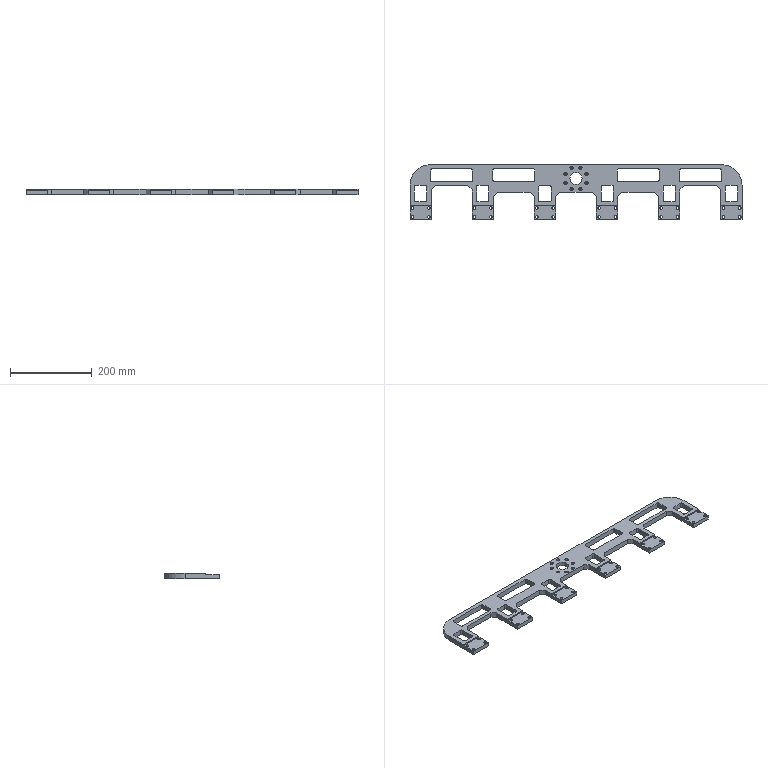NC program | NX | posted with a generic post | part box 813.6 x 134 x 13 mm
Lines 122 to 1368 of 13853:
(ZLEVEL_PROFILE_COPY_3 , TOOL : D10)
N224 T10 M6
N226 G54
N228 G17 G0 G90 X-398.182 Y53.372 S9500 M3
N230 G43 Z30. H10
N232 Z1.5
N234 G94 G1 X-396.786 Y54.924 Z1.391 F1000.
N236 X-394.726 Y56.984 Z1.238
N238 X-392.561 Y58.932 Z1.085
N240 X-390.296 Y60.762 Z0.933
N242 X-387.937 Y62.471 Z0.78
N244 X-385.492 Y64.052 Z0.627
N246 X-382.966 Y65.502 Z0.475
N248 X-380.367 Y66.817 Z0.322
N250 X-377.703 Y67.992 Z0.17
N252 X-374.98 Y69.025 Z0.017
N254 X-372.206 Y69.913 Z-0.136
N256 X-369.389 Y70.653 Z-0.288
N258 X-366.538 Y71.243 Z-0.441
N260 X-363.658 Y71.682 Z-0.594
N262 X-360.76 Y71.968 Z-0.746
N264 X-357.851 Y72.1 Z-0.899
N266 X-356.801 Z-0.954
N268 X356.8 F3500.
N270 G2 X411.9 Y17. R55.1
N272 G1 Y-67.
N274 G2 X406.8 Y-72.1 R5.1
N276 G1 X354.8
N278 G2 X349.7 Y-67. R5.1
N280 G1 Y2.888
N282 X342.687 Y9.9
N284 X266.913
N286 X259.9 Y2.888
N288 Y-67.
N290 G2 X254.8 Y-72.1 R5.1
N292 G1 X202.4
N294 G2 X197.3 Y-67. R5.1
N296 G1 Y-13.062
N298 X190.288 Y-6.05
N300 X114.512
N302 X107.5 Y-13.062
N304 Y-67.
N306 G2 X102.4 Y-72.1 R5.1
N308 G1 X50.
N310 G2 X44.9 Y-67. R5.1
N312 G1 Y-13.062
N314 X37.888 Y-6.05
N316 X-37.888
N318 X-44.9 Y-13.062
N320 Y-67.
N322 G2 X-50. Y-72.1 R5.1
N324 G1 X-102.4
N326 G2 X-107.5 Y-67. R5.1
N328 G1 Y-13.062
N330 X-114.512 Y-6.05
N332 X-190.288
N334 X-197.3 Y-13.062
N336 Y-67.
N338 G2 X-202.4 Y-72.1 R5.1
N340 G1 X-254.8
N342 G2 X-259.9 Y-67. R5.1
N344 G1 Y2.888
N346 X-266.913 Y9.9
N348 X-342.687
N350 X-349.7 Y2.888
N352 Y-67.
N354 G2 X-354.8 Y-72.1 R5.1
N356 G1 X-406.8
N358 G2 X-411.9 Y-67. R5.1
N360 G1 Y16.999
N362 G2 X-356.801 Y72.1 R55.1
N364 G1 X-302.155 Z-1.908
N366 X356.8
N368 G2 X411.9 Y17. R55.1
N370 G1 Y-67.
N372 G2 X406.8 Y-72.1 R5.1
N374 G1 X354.8
N376 G2 X349.7 Y-67. R5.1
N378 G1 Y2.888
N380 X342.687 Y9.9
N382 X266.913
N384 X259.9 Y2.888
N386 Y-67.
N388 G2 X254.8 Y-72.1 R5.1
N390 G1 X202.4
N392 G2 X197.3 Y-67. R5.1
N394 G1 Y-13.062
N396 X190.288 Y-6.05
N398 X114.512
N400 X107.5 Y-13.062
N402 Y-67.
N404 G2 X102.4 Y-72.1 R5.1
N406 G1 X50.
N408 G2 X44.9 Y-67. R5.1
N410 G1 Y-13.062
N412 X37.888 Y-6.05
N414 X-37.888
N416 X-44.9 Y-13.062
N418 Y-67.
N420 G2 X-50. Y-72.1 R5.1
N422 G1 X-102.4
N424 G2 X-107.5 Y-67. R5.1
N426 G1 Y-13.062
N428 X-114.512 Y-6.05
N430 X-190.288
N432 X-197.3 Y-13.062
N434 Y-67.
N436 G2 X-202.4 Y-72.1 R5.1
N438 G1 X-254.8
N440 G2 X-259.9 Y-67. R5.1
N442 G1 Y2.888
N444 X-266.913 Y9.9
N446 X-342.687
N448 X-349.7 Y2.888
N450 Y-67.
N452 G2 X-354.8 Y-72.1 R5.1
N454 G1 X-406.8
N456 G2 X-411.9 Y-67. R5.1
N458 G1 Y16.999
N460 G2 X-356.801 Y72.1 R55.1
N462 G1 X-302.155 Z-2.862
N464 X356.8
N466 G2 X411.9 Y17. R55.1
N468 G1 Y-67.
N470 G2 X406.8 Y-72.1 R5.1
N472 G1 X354.8
N474 G2 X349.7 Y-67. R5.1
N476 G1 Y2.888
N478 X342.687 Y9.9
N480 X266.913
N482 X259.9 Y2.888
N484 Y-67.
N486 G2 X254.8 Y-72.1 R5.1
N488 G1 X202.4
N490 G2 X197.3 Y-67. R5.1
N492 G1 Y-13.062
N494 X190.288 Y-6.05
N496 X114.512
N498 X107.5 Y-13.062
N500 Y-67.
N502 G2 X102.4 Y-72.1 R5.1
N504 G1 X50.
N506 G2 X44.9 Y-67. R5.1
N508 G1 Y-13.062
N510 X37.888 Y-6.05
N512 X-37.888
N514 X-44.9 Y-13.062
N516 Y-67.
N518 G2 X-50. Y-72.1 R5.1
N520 G1 X-102.4
N522 G2 X-107.5 Y-67. R5.1
N524 G1 Y-13.062
N526 X-114.512 Y-6.05
N528 X-190.288
N530 X-197.3 Y-13.062
N532 Y-67.
N534 G2 X-202.4 Y-72.1 R5.1
N536 G1 X-254.8
N538 G2 X-259.9 Y-67. R5.1
N540 G1 Y2.888
N542 X-266.913 Y9.9
N544 X-342.687
N546 X-349.7 Y2.888
N548 Y-67.
N550 G2 X-354.8 Y-72.1 R5.1
N552 G1 X-406.8
N554 G2 X-411.9 Y-67. R5.1
N556 G1 Y16.999
N558 G2 X-356.801 Y72.1 R55.1
N560 G1 X-302.155 Z-3.815
N562 X356.8
N564 G2 X411.9 Y17. R55.1
N566 G1 Y-67.
N568 G2 X406.8 Y-72.1 R5.1
N570 G1 X354.8
N572 G2 X349.7 Y-67. R5.1
N574 G1 Y2.888
N576 X342.687 Y9.9
N578 X266.913
N580 X259.9 Y2.888
N582 Y-67.
N584 G2 X254.8 Y-72.1 R5.1
N586 G1 X202.4
N588 G2 X197.3 Y-67. R5.1
N590 G1 Y-13.062
N592 X190.288 Y-6.05
N594 X114.512
N596 X107.5 Y-13.062
N598 Y-67.
N600 G2 X102.4 Y-72.1 R5.1
N602 G1 X50.
N604 G2 X44.9 Y-67. R5.1
N606 G1 Y-13.062
N608 X37.888 Y-6.05
N610 X-37.888
N612 X-44.9 Y-13.062
N614 Y-67.
N616 G2 X-50. Y-72.1 R5.1
N618 G1 X-102.4
N620 G2 X-107.5 Y-67. R5.1
N622 G1 Y-13.062
N624 X-114.512 Y-6.05
N626 X-190.288
N628 X-197.3 Y-13.062
N630 Y-67.
N632 G2 X-202.4 Y-72.1 R5.1
N634 G1 X-254.8
N636 G2 X-259.9 Y-67. R5.1
N638 G1 Y2.888
N640 X-266.913 Y9.9
N642 X-342.687
N644 X-349.7 Y2.888
N646 Y-67.
N648 G2 X-354.8 Y-72.1 R5.1
N650 G1 X-406.8
N652 G2 X-411.9 Y-67. R5.1
N654 G1 Y16.999
N656 G2 X-356.801 Y72.1 R55.1
N658 G1 X-302.155 Z-4.769
N660 X356.8
N662 G2 X411.9 Y17. R55.1
N664 G1 Y-67.
N666 G2 X406.8 Y-72.1 R5.1
N668 G1 X354.8
N670 G2 X349.7 Y-67. R5.1
N672 G1 Y2.888
N674 X342.687 Y9.9
N676 X266.913
N678 X259.9 Y2.888
N680 Y-67.
N682 G2 X254.8 Y-72.1 R5.1
N684 G1 X202.4
N686 G2 X197.3 Y-67. R5.1
N688 G1 Y-13.062
N690 X190.288 Y-6.05
N692 X114.512
N694 X107.5 Y-13.062
N696 Y-67.
N698 G2 X102.4 Y-72.1 R5.1
N700 G1 X50.
N702 G2 X44.9 Y-67. R5.1
N704 G1 Y-13.062
N706 X37.888 Y-6.05
N708 X-37.888
N710 X-44.9 Y-13.062
N712 Y-67.
N714 G2 X-50. Y-72.1 R5.1
N716 G1 X-102.4
N718 G2 X-107.5 Y-67. R5.1
N720 G1 Y-13.062
N722 X-114.512 Y-6.05
N724 X-190.288
N726 X-197.3 Y-13.062
N728 Y-67.
N730 G2 X-202.4 Y-72.1 R5.1
N732 G1 X-254.8
N734 G2 X-259.9 Y-67. R5.1
N736 G1 Y2.888
N738 X-266.913 Y9.9
N740 X-342.687
N742 X-349.7 Y2.888
N744 Y-67.
N746 G2 X-354.8 Y-72.1 R5.1
N748 G1 X-406.8
N750 G2 X-411.9 Y-67. R5.1
N752 G1 Y16.999
N754 G2 X-356.801 Y72.1 R55.1
N756 G1 X-302.155 Z-5.723
N758 X356.8
N760 G2 X411.9 Y17. R55.1
N762 G1 Y-67.
N764 G2 X406.8 Y-72.1 R5.1
N766 G1 X354.8
N768 G2 X349.7 Y-67. R5.1
N770 G1 Y2.888
N772 X342.687 Y9.9
N774 X266.913
N776 X259.9 Y2.888
N778 Y-67.
N780 G2 X254.8 Y-72.1 R5.1
N782 G1 X202.4
N784 G2 X197.3 Y-67. R5.1
N786 G1 Y-13.062
N788 X190.288 Y-6.05
N790 X114.512
N792 X107.5 Y-13.062
N794 Y-67.
N796 G2 X102.4 Y-72.1 R5.1
N798 G1 X50.
N800 G2 X44.9 Y-67. R5.1
N802 G1 Y-13.062
N804 X37.888 Y-6.05
N806 X-37.888
N808 X-44.9 Y-13.062
N810 Y-67.
N812 G2 X-50. Y-72.1 R5.1
N814 G1 X-102.4
N816 G2 X-107.5 Y-67. R5.1
N818 G1 Y-13.062
N820 X-114.512 Y-6.05
N822 X-190.288
N824 X-197.3 Y-13.062
N826 Y-67.
N828 G2 X-202.4 Y-72.1 R5.1
N830 G1 X-254.8
N832 G2 X-259.9 Y-67. R5.1
N834 G1 Y2.888
N836 X-266.913 Y9.9
N838 X-342.687
N840 X-349.7 Y2.888
N842 Y-67.
N844 G2 X-354.8 Y-72.1 R5.1
N846 G1 X-406.8
N848 G2 X-411.9 Y-67. R5.1
N850 G1 Y16.999
N852 G2 X-356.801 Y72.1 R55.1
N854 G1 X-302.155 Z-6.677
N856 X356.8
N858 G2 X411.9 Y17. R55.1
N860 G1 Y-67.
N862 G2 X406.8 Y-72.1 R5.1
N864 G1 X354.8
N866 G2 X349.7 Y-67. R5.1
N868 G1 Y2.888
N870 X342.687 Y9.9
N872 X266.913
N874 X259.9 Y2.888
N876 Y-67.
N878 G2 X254.8 Y-72.1 R5.1
N880 G1 X202.4
N882 G2 X197.3 Y-67. R5.1
N884 G1 Y-13.062
N886 X190.288 Y-6.05
N888 X114.512
N890 X107.5 Y-13.062
N892 Y-67.
N894 G2 X102.4 Y-72.1 R5.1
N896 G1 X50.
N898 G2 X44.9 Y-67. R5.1
N900 G1 Y-13.062
N902 X37.888 Y-6.05
N904 X-37.888
N906 X-44.9 Y-13.062
N908 Y-67.
N910 G2 X-50. Y-72.1 R5.1
N912 G1 X-102.4
N914 G2 X-107.5 Y-67. R5.1
N916 G1 Y-13.062
N918 X-114.512 Y-6.05
N920 X-190.288
N922 X-197.3 Y-13.062
N924 Y-67.
N926 G2 X-202.4 Y-72.1 R5.1
N928 G1 X-254.8
N930 G2 X-259.9 Y-67. R5.1
N932 G1 Y2.888
N934 X-266.913 Y9.9
N936 X-342.687
N938 X-349.7 Y2.888
N940 Y-67.
N942 G2 X-354.8 Y-72.1 R5.1
N944 G1 X-406.8
N946 G2 X-411.9 Y-67. R5.1
N948 G1 Y16.999
N950 G2 X-356.801 Y72.1 R55.1
N952 G1 X-302.155 Z-7.631
N954 X356.8
N956 G2 X411.9 Y17. R55.1
N958 G1 Y-67.
N960 G2 X406.8 Y-72.1 R5.1
N962 G1 X354.8
N964 G2 X349.7 Y-67. R5.1
N966 G1 Y2.888
N968 X342.687 Y9.9
N970 X266.913
N972 X259.9 Y2.888
N974 Y-67.
N976 G2 X254.8 Y-72.1 R5.1
N978 G1 X202.4
N980 G2 X197.3 Y-67. R5.1
N982 G1 Y-13.062
N984 X190.288 Y-6.05
N986 X114.512
N988 X107.5 Y-13.062
N990 Y-67.
N992 G2 X102.4 Y-72.1 R5.1
N994 G1 X50.
N996 G2 X44.9 Y-67. R5.1
N998 G1 Y-13.062
N1000 X37.888 Y-6.05
N1002 X-37.888
N1004 X-44.9 Y-13.062
N1006 Y-67.
N1008 G2 X-50. Y-72.1 R5.1
N1010 G1 X-102.4
N1012 G2 X-107.5 Y-67. R5.1
N1014 G1 Y-13.062
N1016 X-114.512 Y-6.05
N1018 X-190.288
N1020 X-197.3 Y-13.062
N1022 Y-67.
N1024 G2 X-202.4 Y-72.1 R5.1
N1026 G1 X-254.8
N1028 G2 X-259.9 Y-67. R5.1
N1030 G1 Y2.888
N1032 X-266.913 Y9.9
N1034 X-342.687
N1036 X-349.7 Y2.888
N1038 Y-67.
N1040 G2 X-354.8 Y-72.1 R5.1
N1042 G1 X-406.8
N1044 G2 X-411.9 Y-67. R5.1
N1046 G1 Y16.999
N1048 G2 X-356.801 Y72.1 R55.1
N1050 G1 X-302.377 Z-8.581
N1052 X-302.155 Z-8.585
N1054 X356.8
N1056 G2 X411.9 Y17. R55.1
N1058 G1 Y-67.
N1060 G2 X406.8 Y-72.1 R5.1
N1062 G1 X354.8
N1064 G2 X349.7 Y-67. R5.1
N1066 G1 Y2.888
N1068 X342.688 Y9.9
N1070 X266.912
N1072 X259.9 Y2.888
N1074 Y-67.
N1076 G2 X254.8 Y-72.1 R5.1
N1078 G1 X202.4
N1080 G2 X197.3 Y-67. R5.1
N1082 G1 Y-13.062
N1084 X190.288 Y-6.05
N1086 X114.512
N1088 X107.5 Y-13.062
N1090 Y-67.
N1092 G2 X102.4 Y-72.1 R5.1
N1094 G1 X50.
N1096 G2 X44.9 Y-67. R5.1
N1098 G1 Y-13.062
N1100 X37.888 Y-6.05
N1102 X-37.888
N1104 X-44.9 Y-13.062
N1106 Y-67.
N1108 G2 X-50. Y-72.1 R5.1
N1110 G1 X-102.4
N1112 G2 X-107.5 Y-67. R5.1
N1114 G1 Y-13.062
N1116 X-114.512 Y-6.05
N1118 X-190.288
N1120 X-197.3 Y-13.062
N1122 Y-67.
N1124 G2 X-202.4 Y-72.1 R5.1
N1126 G1 X-254.8
N1128 G2 X-259.9 Y-67. R5.1
N1130 G1 Y2.888
N1132 X-266.912 Y9.9
N1134 X-342.688
N1136 X-349.7 Y2.888
N1138 Y-67.
N1140 G2 X-354.8 Y-72.1 R5.1
N1142 G1 X-406.8
N1144 G2 X-411.9 Y-67. R5.1
N1146 G1 Y16.999
N1148 G2 X-356.801 Y72.1 R55.1
N1150 G1 X-356.579 Z-8.588
N1152 X-302.377 Z-9.535
N1154 X-302.155 Z-9.538
N1156 X356.8
N1158 G2 X411.9 Y17. R55.1
N1160 G1 Y-67.
N1162 G2 X406.8 Y-72.1 R5.1
N1164 G1 X354.8
N1166 G2 X349.7 Y-67. R5.1
N1168 G1 Y2.888
N1170 X342.688 Y9.9
N1172 X266.912
N1174 X259.9 Y2.888
N1176 Y-67.
N1178 G2 X254.8 Y-72.1 R5.1
N1180 G1 X202.4
N1182 G2 X197.3 Y-67. R5.1
N1184 G1 Y-13.062
N1186 X190.288 Y-6.05
N1188 X114.512
N1190 X107.5 Y-13.062
N1192 Y-67.
N1194 G2 X102.4 Y-72.1 R5.1
N1196 G1 X50.
N1198 G2 X44.9 Y-67. R5.1
N1200 G1 Y-13.062
N1202 X37.888 Y-6.05
N1204 X-37.888
N1206 X-44.9 Y-13.062
N1208 Y-67.
N1210 G2 X-50. Y-72.1 R5.1
N1212 G1 X-102.4
N1214 G2 X-107.5 Y-67. R5.1
N1216 G1 Y-13.062
N1218 X-114.512 Y-6.05
N1220 X-190.288
N1222 X-197.3 Y-13.062
N1224 Y-67.
N1226 G2 X-202.4 Y-72.1 R5.1
N1228 G1 X-254.8
N1230 G2 X-259.9 Y-67. R5.1
N1232 G1 Y2.888
N1234 X-266.912 Y9.9
N1236 X-342.688
N1238 X-349.7 Y2.888
N1240 Y-67.
N1242 G2 X-354.8 Y-72.1 R5.1
N1244 G1 X-406.8
N1246 G2 X-411.9 Y-67. R5.1
N1248 G1 Y16.999
N1250 G2 X-356.801 Y72.1 R55.1
N1252 G1 X-356.579 Z-9.542
N1254 X-302.377 Z-10.488
N1256 X-302.155 Z-10.492
N1258 X356.8
N1260 G2 X411.9 Y17. R55.1
N1262 G1 Y-67.
N1264 G2 X406.8 Y-72.1 R5.1
N1266 G1 X354.8
N1268 G2 X349.7 Y-67. R5.1
N1270 G1 Y2.888
N1272 X342.688 Y9.9
N1274 X266.912
N1276 X259.9 Y2.888
N1278 Y-67.
N1280 G2 X254.8 Y-72.1 R5.1
N1282 G1 X202.4
N1284 G2 X197.3 Y-67. R5.1
N1286 G1 Y-13.062
N1288 X190.288 Y-6.05
N1290 X114.512
N1292 X107.5 Y-13.062
N1294 Y-67.
N1296 G2 X102.4 Y-72.1 R5.1
N1298 G1 X50.
N1300 G2 X44.9 Y-67. R5.1
N1302 G1 Y-13.062
N1304 X37.888 Y-6.05
N1306 X-37.888
N1308 X-44.9 Y-13.062
N1310 Y-67.
N1312 G2 X-50. Y-72.1 R5.1
N1314 G1 X-102.4
N1316 G2 X-107.5 Y-67. R5.1
N1318 G1 Y-13.062
N1320 X-114.512 Y-6.05
N1322 X-190.288
N1324 X-197.3 Y-13.062
N1326 Y-67.
N1328 G2 X-202.4 Y-72.1 R5.1
N1330 G1 X-254.8
N1332 G2 X-259.9 Y-67. R5.1
N1334 G1 Y2.888
N1336 X-266.912 Y9.9
N1338 X-342.688
N1340 X-349.7 Y2.888
N1342 Y-67.
N1344 G2 X-354.8 Y-72.1 R5.1
N1346 G1 X-406.8
N1348 G2 X-411.9 Y-67. R5.1
N1350 G1 Y16.999
N1352 G2 X-356.801 Y72.1 R55.1
N1354 G1 X-356.579 Z-10.496
N1356 X-302.377 Z-11.442
N1358 X-302.155 Z-11.446
N1360 X356.8
N1362 G2 X411.9 Y17. R55.1
N1364 G1 Y-67.
N1366 G2 X406.8 Y-72.1 R5.1
N1368 G1 X354.8
N1370 G2 X349.7 Y-67. R5.1
N1372 G1 Y2.888
N1374 X342.688 Y9.9
N1376 X266.912
N1378 X259.9 Y2.888
N1380 Y-67.
N1382 G2 X254.8 Y-72.1 R5.1
N1384 G1 X202.4
N1386 G2 X197.3 Y-67. R5.1
N1388 G1 Y-13.062
N1390 X190.288 Y-6.05
N1392 X114.512
N1394 X107.5 Y-13.062
N1396 Y-67.
N1398 G2 X102.4 Y-72.1 R5.1
N1400 G1 X50.
N1402 G2 X44.9 Y-67. R5.1
N1404 G1 Y-13.062
N1406 X37.888 Y-6.05
N1408 X-37.888
N1410 X-44.9 Y-13.062
N1412 Y-67.
N1414 G2 X-50. Y-72.1 R5.1
N1416 G1 X-102.4
N1418 G2 X-107.5 Y-67. R5.1
N1420 G1 Y-13.062
N1422 X-114.512 Y-6.05
N1424 X-190.288
N1426 X-197.3 Y-13.062
N1428 Y-67.
N1430 G2 X-202.4 Y-72.1 R5.1
N1432 G1 X-254.8
N1434 G2 X-259.9 Y-67. R5.1
N1436 G1 Y2.888
N1438 X-266.912 Y9.9
N1440 X-342.688
N1442 X-349.7 Y2.888
N1444 Y-67.
N1446 G2 X-354.8 Y-72.1 R5.1
N1448 G1 X-406.8
N1450 G2 X-411.9 Y-67. R5.1
N1452 G1 Y16.999
N1454 G2 X-356.801 Y72.1 R55.1
N1456 G1 X-356.579 Z-11.45
N1458 X-302.377 Z-12.396
N1460 X-302.155 Z-12.4
N1462 X356.8
N1464 G2 X411.9 Y17. R55.1
N1466 G1 Y-67.
N1468 G2 X406.8 Y-72.1 R5.1
N1470 G1 X354.8
N1472 G2 X349.7 Y-67. R5.1
N1474 G1 Y2.888
N1476 X342.688 Y9.9
N1478 X266.912
N1480 X259.9 Y2.888
N1482 Y-67.
N1484 G2 X254.8 Y-72.1 R5.1
N1486 G1 X202.4
N1488 G2 X197.3 Y-67. R5.1
N1490 G1 Y-13.062
N1492 X190.288 Y-6.05
N1494 X114.512
N1496 X107.5 Y-13.062
N1498 Y-67.
N1500 G2 X102.4 Y-72.1 R5.1
N1502 G1 X50.
N1504 G2 X44.9 Y-67. R5.1
N1506 G1 Y-13.062
N1508 X37.888 Y-6.05
N1510 X-37.888
N1512 X-44.9 Y-13.062
N1514 Y-67.
N1516 G2 X-50. Y-72.1 R5.1
N1518 G1 X-102.4
N1520 G2 X-107.5 Y-67. R5.1
N1522 G1 Y-13.062
N1524 X-114.512 Y-6.05
N1526 X-190.288
N1528 X-197.3 Y-13.062
N1530 Y-67.
N1532 G2 X-202.4 Y-72.1 R5.1
N1534 G1 X-254.8
N1536 G2 X-259.9 Y-67. R5.1
N1538 G1 Y2.888
N1540 X-266.912 Y9.9
N1542 X-342.688
N1544 X-349.7 Y2.888
N1546 Y-67.
N1548 G2 X-354.8 Y-72.1 R5.1
N1550 G1 X-406.8
N1552 G2 X-411.9 Y-67. R5.1
N1554 G1 Y16.999
N1556 G2 X-356.801 Y72.1 R55.1
N1558 G1 X-302.155
N1560 Z-10.9
N1562 G0 Z30.
(ZLEVEL_PROFILE_COPY_2_COPY , TOOL : D10)
N1564 X350.7 Y50.247
N1566 Z1.5
N1568 G1 Y51.903 Z1.413 F1000.
N1570 X350.663 Y51.9 Z1.411
N1572 X304.8 Z-0.992
N1574 X258.94 F3500.
N1576 X258.9 Y51.903
N1578 Y30.1
N1580 X350.7
N1582 Y51.903
N1584 X350.663 Y51.9
N1586 X304.8
N1588 X259.054 Z-1.791
N1590 X258.9 Z-1.794
N1592 Y51.613 Z-1.799
N1594 Y40.954 Z-1.985
N1596 Y30.1
N1598 X350.7
N1600 Y51.903
N1602 X350.663 Y51.9
N1604 X304.8
N1606 X259.054 Z-2.783
N1608 X258.9 Z-2.786
N1610 Y51.613 Z-2.791
N1612 Y40.953 Z-2.977
N1614 Y30.1
N1616 X350.7
N1618 Y51.903
N1620 X350.663 Y51.9
N1622 X304.8
N1624 X259.054 Z-3.775
N1626 X258.9 Z-3.778
N1628 Y51.613 Z-3.783
N1630 Y40.953 Z-3.969
N1632 Y30.1
N1634 X350.7
N1636 Y51.903
N1638 X350.663 Y51.9
N1640 X304.8
N1642 X259.054 Z-4.768
N1644 X258.9 Z-4.77
N1646 Y51.613 Z-4.775
N1648 Y40.953 Z-4.962
N1650 Y30.1
N1652 X350.7
N1654 Y51.903
N1656 X350.663 Y51.9
N1658 X304.8
N1660 X259.054 Z-5.76
N1662 X258.9 Z-5.763
N1664 Y51.613 Z-5.768
N1666 Y40.953 Z-5.954
N1668 Y30.1
N1670 X350.7
N1672 Y51.903
N1674 X350.663 Y51.9
N1676 X304.8
N1678 X259.054 Z-6.752
N1680 X258.9 Z-6.755
N1682 Y51.613 Z-6.76
N1684 Y40.953 Z-6.946
N1686 Y30.1
N1688 X350.7
N1690 Y51.903
N1692 X350.663 Y51.9
N1694 X304.8
N1696 X259.054 Z-7.745
N1698 X258.9 Z-7.747
N1700 Y51.613 Z-7.752
N1702 Y40.953 Z-7.938
N1704 Y30.1
N1706 X350.7
N1708 Y51.903
N1710 X350.663 Y51.9
N1712 X304.8
N1714 X259.054 Z-8.737
N1716 X258.9 Z-8.74
N1718 Y51.613 Z-8.745
N1720 Y40.953 Z-8.931
N1722 Y30.1
N1724 X350.7
N1726 Y51.903
N1728 X350.663 Y51.9
N1730 X304.8
N1732 X259.054 Z-9.729
N1734 X258.9 Z-9.732
N1736 Y51.613 Z-9.737
N1738 Y40.953 Z-9.923
N1740 Y30.1
N1742 X350.7
N1744 Y51.903
N1746 X350.663 Y51.9
N1748 X304.8
N1750 X259.054 Z-10.722
N1752 X258.9 Z-10.724
N1754 Y51.613 Z-10.729
N1756 Y40.953 Z-10.915
N1758 Y30.1
N1760 X350.7
N1762 Y51.903
N1764 X350.663 Y51.9
N1766 X304.8
N1768 X259.054 Z-11.714
N1770 X258.9 Z-11.717
N1772 Y51.613 Z-11.722
N1774 Y40.953 Z-11.908
N1776 Y30.1
N1778 X350.7
N1780 Y51.903
N1782 X350.663 Y51.9
N1784 X304.8
N1786 X259.054 Z-12.706
N1788 X258.9 Z-12.709
N1790 Y51.613 Z-12.714
N1792 Y40.953 Z-12.9
N1794 Y30.1
N1796 X350.7
N1798 Y51.903
N1800 X350.663 Y51.9
N1802 X258.94
N1804 X258.9 Y51.903
N1806 Y40.953
N1808 Z-11.4
N1810 G0 Z30.
N1812 X198.3 Y50.246
N1814 Z1.5
N1816 G1 Y51.902 Z1.413 F1000.
N1818 X198.262 Y51.9 Z1.411
N1820 X152.4 Z-0.992
N1822 X106.539 F3500.
N1824 X106.5 Y51.902
N1826 Y30.1
N1828 X198.3
N1830 Y51.902
N1832 X198.262 Y51.9
N1834 X152.4
N1836 X106.654 Z-1.791
N1838 X106.5 Z-1.794
N1840 Y51.612 Z-1.799
N1842 Y40.953 Z-1.985
N1844 Y30.1
N1846 X198.3
N1848 Y51.902
N1850 X198.262 Y51.9
N1852 X152.4
N1854 X106.654 Z-2.783
N1856 X106.5 Z-2.786
N1858 Y51.612 Z-2.791
N1860 Y40.953 Z-2.977
N1862 Y30.1
N1864 X198.3
N1866 Y51.902
N1868 X198.262 Y51.9
N1870 X152.4
N1872 X106.654 Z-3.775
N1874 X106.5 Z-3.778
N1876 Y51.612 Z-3.783
N1878 Y40.953 Z-3.969
N1880 Y30.1
N1882 X198.3
N1884 Y51.902
N1886 X198.262 Y51.9
N1888 X152.4
N1890 X106.654 Z-4.768
N1892 X106.5 Z-4.77
N1894 Y51.612 Z-4.775
N1896 Y40.953 Z-4.962
N1898 Y30.1
N1900 X198.3
N1902 Y51.902
N1904 X198.262 Y51.9
N1906 X152.4
N1908 X106.654 Z-5.76
N1910 X106.5 Z-5.763
N1912 Y51.612 Z-5.768
N1914 Y40.953 Z-5.954
N1916 Y30.1
N1918 X198.3
N1920 Y51.902
N1922 X198.262 Y51.9
N1924 X152.4
N1926 X106.654 Z-6.752
N1928 X106.5 Z-6.755
N1930 Y51.612 Z-6.76
N1932 Y40.953 Z-6.946
N1934 Y30.1
N1936 X198.3
N1938 Y51.902
N1940 X198.262 Y51.9
N1942 X152.4
N1944 X106.654 Z-7.745
N1946 X106.5 Z-7.747
N1948 Y51.612 Z-7.752
N1950 Y40.953 Z-7.938
N1952 Y30.1
N1954 X198.3
N1956 Y51.902
N1958 X198.262 Y51.9
N1960 X152.4
N1962 X106.654 Z-8.737
N1964 X106.5 Z-8.74
N1966 Y51.612 Z-8.745
N1968 Y40.953 Z-8.931
N1970 Y30.1
N1972 X198.3
N1974 Y51.902
N1976 X198.262 Y51.9
N1978 X152.4
N1980 X106.654 Z-9.729
N1982 X106.5 Z-9.732
N1984 Y51.612 Z-9.737
N1986 Y40.953 Z-9.923
N1988 Y30.1
N1990 X198.3
N1992 Y51.902
N1994 X198.262 Y51.9
N1996 X152.4
N1998 X106.654 Z-10.722
N2000 X106.5 Z-10.724
N2002 Y51.612 Z-10.729
N2004 Y40.953 Z-10.915
N2006 Y30.1
N2008 X198.3
N2010 Y51.902
N2012 X198.262 Y51.9
N2014 X152.4
N2016 X106.654 Z-11.714
N2018 X106.5 Z-11.717
N2020 Y51.612 Z-11.722
N2022 Y40.953 Z-11.908
N2024 Y30.1
N2026 X198.3
N2028 Y51.902
N2030 X198.262 Y51.9
N2032 X152.4
N2034 X106.654 Z-12.706
N2036 X106.5 Z-12.709
N2038 Y51.612 Z-12.714
N2040 Y40.953 Z-12.9
N2042 Y30.1
N2044 X198.3
N2046 Y51.902
N2048 X198.262 Y51.9
N2050 X106.539
N2052 X106.5 Y51.902
N2054 Y40.953
N2056 Z-11.4
N2058 G0 Z30.
N2060 X371.3 Y-6.045
N2062 Z1.5
N2064 G1 Y-18.9 Z0.826 F1000.
N2066 X391.1 Z-0.211
N2068 Y-3.999 Z-0.992
N2070 Y10.902 F3500.
N2072 X391.053 Y10.9
N2074 X371.3
N2076 Y-18.9
N2078 X391.1
N2080 Y-3.999
N2082 Y10.657 Z-1.248
N2084 Y10.9 Z-1.252
N2086 X390.9 Z-1.256
N2088 X371.3 Z-1.598
N2090 Y-11.248 Z-1.985
N2092 Y-18.9
N2094 X391.1
N2096 Y-3.999
N2098 Y10.657 Z-2.24
N2100 Y10.9 Z-2.245
N2102 X390.9 Z-2.248
N2104 X371.3 Z-2.59
N2106 Y-11.248 Z-2.977
N2108 Y-18.9
N2110 X391.1
N2112 Y-3.999
N2114 Y10.657 Z-3.233
N2116 Y10.9 Z-3.237
N2118 X390.9 Z-3.241
N2120 X371.3 Z-3.583
N2122 Y-11.248 Z-3.969
N2124 Y-18.9
N2126 X391.1
N2128 Y-3.999
N2130 Y10.657 Z-4.225
N2132 Y10.9 Z-4.229
N2134 X390.9 Z-4.233
N2136 X371.3 Z-4.575
N2138 Y-11.248 Z-4.962
N2140 Y-18.9
N2142 X391.1
N2144 Y-3.999
N2146 Y10.657 Z-5.217
N2148 Y10.9 Z-5.222
N2150 X390.9 Z-5.225
N2152 X371.3 Z-5.567
N2154 Y-11.248 Z-5.954
N2156 Y-18.9
N2158 X391.1
N2160 Y-3.999
N2162 Y10.657 Z-6.21
N2164 Y10.9 Z-6.214
N2166 X390.9 Z-6.217
N2168 X371.3 Z-6.56
N2170 Y-11.248 Z-6.946
N2172 Y-18.9
N2174 X391.1
N2176 Y-3.999
N2178 Y10.657 Z-7.202
N2180 Y10.9 Z-7.206
N2182 X390.9 Z-7.21
N2184 X371.3 Z-7.552
N2186 Y-11.248 Z-7.938
N2188 Y-18.9
N2190 X391.1
N2192 Y-3.999
N2194 Y10.657 Z-8.194
N2196 Y10.9 Z-8.199
N2198 X390.9 Z-8.202
N2200 X371.3 Z-8.544
N2202 Y-11.248 Z-8.931
N2204 Y-18.9
N2206 X391.1
N2208 Y-3.999
N2210 Y10.657 Z-9.187
N2212 Y10.9 Z-9.191
N2214 X390.9 Z-9.194
N2216 X371.3 Z-9.536
N2218 Y-11.248 Z-9.923
N2220 Y-18.9
N2222 X391.1
N2224 Y-3.999
N2226 Y10.657 Z-10.179
N2228 Y10.9 Z-10.183
N2230 X390.9 Z-10.187
N2232 X371.3 Z-10.529
N2234 Y-11.248 Z-10.915
N2236 Y-18.9
N2238 X391.1
N2240 Y-3.999
N2242 Y10.657 Z-11.171
N2244 Y10.9 Z-11.175
N2246 X390.9 Z-11.179
N2248 X371.3 Z-11.521
N2250 Y-11.248 Z-11.908
N2252 Y-18.9
N2254 X391.1
N2256 Y-3.999
N2258 Y10.657 Z-12.164
N2260 Y10.9 Z-12.168
N2262 X390.9 Z-12.171
N2264 X371.3 Z-12.513
N2266 Y-11.248 Z-12.9
N2268 Y-18.9
N2270 X391.1
N2272 Y10.902
N2274 X391.053 Y10.9
N2276 X371.3
N2278 Y-11.248
N2280 Z-11.4
N2282 G0 Z30.
N2284 X218.9 Y-6.045
N2286 Z1.5
N2288 G1 Y-18.9 Z0.826 F1000.
N2290 X238.7 Z-0.211
N2292 Y-3.999 Z-0.992
N2294 Y10.902 F3500.
N2296 X238.653 Y10.9
N2298 X218.947
N2300 X218.9 Y10.902
N2302 Y-18.9
N2304 X238.7
N2306 Y-3.999
N2308 Y10.657 Z-1.248
N2310 Y10.9 Z-1.252
N2312 X238.5 Z-1.256
N2314 X218.959 Z-1.597
N2316 X218.9 Z-1.598
N2318 Y10.516 Z-1.605
N2320 Y-11.246 Z-1.985
N2322 Y-18.9
N2324 X238.7
N2326 Y-3.999
N2328 Y10.657 Z-2.24
N2330 Y10.9 Z-2.245
N2332 X238.5 Z-2.248
N2334 X218.959 Z-2.589
N2336 X218.9 Z-2.59
N2338 Y10.516 Z-2.597
N2340 Y-11.246 Z-2.977
N2342 Y-18.9
N2344 X238.7
N2346 Y-3.999
N2348 Y10.657 Z-3.233
N2350 Y10.9 Z-3.237
N2352 X238.5 Z-3.241
N2354 X218.958 Z-3.582
N2356 X218.9 Z-3.583
N2358 Y10.516 Z-3.589
N2360 Y-11.246 Z-3.969
N2362 Y-18.9
N2364 X238.7
N2366 Y-3.999
N2368 Y10.657 Z-4.225
N2370 Y10.9 Z-4.229
N2372 X238.5 Z-4.233
N2374 X218.958 Z-4.574
N2376 X218.9 Z-4.575
N2378 Y10.516 Z-4.582
N2380 Y-11.246 Z-4.962
N2382 Y-18.9
N2384 X238.7
N2386 Y-3.999
N2388 Y10.657 Z-5.217
N2390 Y10.9 Z-5.222
N2392 X238.5 Z-5.225
N2394 X218.958 Z-5.566
N2396 X218.9 Z-5.567
N2398 Y10.516 Z-5.574
N2400 Y-11.246 Z-5.954
N2402 Y-18.9
N2404 X238.7
N2406 Y-3.999
N2408 Y10.657 Z-6.21
N2410 Y10.9 Z-6.214
N2412 X238.5 Z-6.217
N2414 X218.958 Z-6.559
N2416 X218.9 Z-6.56
N2418 Y10.516 Z-6.566
N2420 Y-11.246 Z-6.946
N2422 Y-18.9
N2424 X238.7
N2426 Y-3.999
N2428 Y10.657 Z-7.202
N2430 Y10.9 Z-7.206
N2432 X238.5 Z-7.21
N2434 X218.958 Z-7.551
N2436 X218.9 Z-7.552
N2438 Y10.516 Z-7.559
N2440 Y-11.246 Z-7.938
N2442 Y-18.9
N2444 X238.7
N2446 Y-3.999
N2448 Y10.657 Z-8.194
N2450 Y10.9 Z-8.199
N2452 X238.5 Z-8.202
N2454 X218.958 Z-8.543
N2456 X218.9 Z-8.544
N2458 Y10.516 Z-8.551
N2460 Y-11.246 Z-8.931
N2462 Y-18.9
N2464 X238.7
N2466 Y-3.999
N2468 Y10.657 Z-9.187
N2470 Y10.9 Z-9.191
N2472 X238.5 Z-9.194
N2474 X218.958 Z-9.535
N2476 X218.9 Z-9.536
N2478 Y10.516 Z-9.543
N2480 Y-11.246 Z-9.923
N2482 Y-18.9
N2484 X238.7
N2486 Y-3.999
N2488 Y10.657 Z-10.179
N2490 Y10.9 Z-10.183
N2492 X238.5 Z-10.187
N2494 X218.958 Z-10.528
N2496 X218.9 Z-10.529
N2498 Y10.516 Z-10.536
N2500 Y-11.246 Z-10.915
N2502 Y-18.9
N2504 X238.7
N2506 Y-3.999
N2508 Y10.657 Z-11.171
N2510 Y10.9 Z-11.175
N2512 X238.5 Z-11.179
N2514 X218.958 Z-11.52
N2516 X218.9 Z-11.521
N2518 Y10.516 Z-11.528
N2520 Y-11.246 Z-11.908
N2522 Y-18.9
N2524 X238.7
N2526 Y-3.999
N2528 Y10.657 Z-12.164
N2530 Y10.9 Z-12.168
N2532 X238.5 Z-12.171
N2534 X218.958 Z-12.512
N2536 X218.9 Z-12.513
N2538 Y10.516 Z-12.52
N2540 Y-11.246 Z-12.9
N2542 Y-18.9
N2544 X238.7
N2546 Y10.902
N2548 X238.653 Y10.9
N2550 X218.947
N2552 X218.9 Y10.902
N2554 Y-11.246
N2556 Z-11.4
N2558 G0 Z30.
N2560 X66.5 Y-6.044
N2562 Z1.5
N2564 G1 Y-18.9 Z0.826 F1000.
N2566 X86.3 Z-0.211
N2568 Y-4. Z-0.992
N2570 Y10.9 F3500.
N2572 X66.547
N2574 X66.5 Y10.902
N2576 Y-18.9
N2578 X86.3
N2580 Y-4.
N2582 Y10.9 Z-1.252
N2584 X66.557 Z-1.597
N2586 X66.5 Z-1.598
N2588 Y10.515 Z-1.605
N2590 Y-11.248 Z-1.985
N2592 Y-18.9
N2594 X86.3
N2596 Y-4.
N2598 Y10.9 Z-2.245
N2600 X66.557 Z-2.589
N2602 X66.5 Z-2.59
N2604 Y10.515 Z-2.597
N2606 Y-11.248 Z-2.977
N2608 Y-18.9
N2610 X86.3
N2612 Y-4.
N2614 Y10.9 Z-3.237
N2616 X66.557 Z-3.582
N2618 X66.5 Z-3.583
N2620 Y10.515 Z-3.589
N2622 Y-11.248 Z-3.969
N2624 Y-18.9
N2626 X86.3
N2628 Y-4.
N2630 Y10.9 Z-4.229
N2632 X66.557 Z-4.574
N2634 X66.5 Z-4.575
N2636 Y10.515 Z-4.582
N2638 Y-11.248 Z-4.962
N2640 Y-18.9
N2642 X86.3
N2644 Y-4.
N2646 Y10.9 Z-5.222
N2648 X66.557 Z-5.566
N2650 X66.5 Z-5.567
N2652 Y10.515 Z-5.574
N2654 Y-11.248 Z-5.954
N2656 Y-18.9
N2658 X86.3
N2660 Y-4.
N2662 Y10.9 Z-6.214
N2664 X66.557 Z-6.559
N2666 X66.5 Z-6.56
N2668 Y10.515 Z-6.566
N2670 Y-11.248 Z-6.946
N2672 Y-18.9
N2674 X86.3
N2676 Y-4.
N2678 Y10.9 Z-7.206
N2680 X66.557 Z-7.551
N2682 X66.5 Z-7.552
N2684 Y10.515 Z-7.559
N2686 Y-11.248 Z-7.938
N2688 Y-18.9
N2690 X86.3
N2692 Y-4.
N2694 Y10.9 Z-8.199
N2696 X66.557 Z-8.543
N2698 X66.5 Z-8.544
N2700 Y10.515 Z-8.551
N2702 Y-11.248 Z-8.931
N2704 Y-18.9